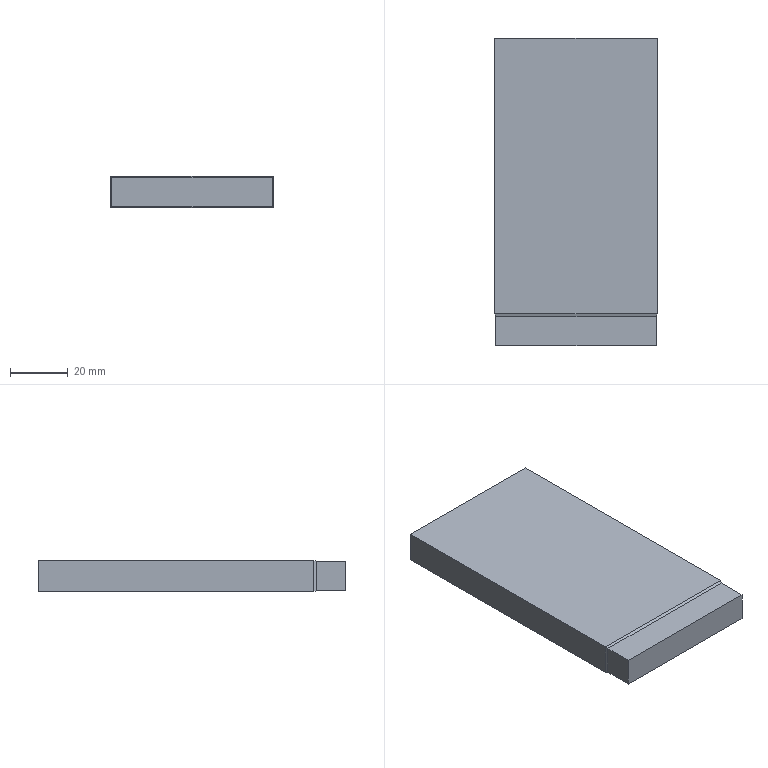Part | STEP file | 1 solid | 14 faces | box 56.208 x 106.38 x 10.782 mm | volume 63955 mm3 | plane 14
STEP:
#1=CARTESIAN_POINT('',(0.,0.,0.));
#2=DIRECTION('',(0.,0.,1.));
#3=DIRECTION('',(1.,0.,0.));
#4=AXIS2_PLACEMENT_3D('',#1,#2,#3);
#5=CARTESIAN_POINT('',(-93.931,130.5,161.754));
#6=VERTEX_POINT('',#5);
#7=CARTESIAN_POINT('',(-93.931,35.175,161.754));
#8=VERTEX_POINT('',#7);
#9=CARTESIAN_POINT('',(-93.931,185.175,161.754));
#10=DIRECTION('',(0.,-1.,0.));
#11=VECTOR('',#10,1.);
#12=LINE('',#9,#11);
#13=CARTESIAN_POINT('',(-93.931,185.175,150.972));
#14=DIRECTION('',(1.,0.,0.));
#15=DIRECTION('',(0.,0.,-1.));
#16=AXIS2_PLACEMENT_3D('',#13,#14,#15);
#17=PLANE('',#16);
#18=CARTESIAN_POINT('',(-10.782,0.));
#19=DIRECTION('',(0.,-1.));
#20=VECTOR('',#19,1.);
#21=LINE('',#18,#20);
#22=(GEOMETRIC_REPRESENTATION_CONTEXT(2)PARAMETRIC_REPRESENTATION_CONTEXT()REPRESENTATION_CONTEXT('',''));
#23=DEFINITIONAL_REPRESENTATION('',(#21),#22);
#24=PCURVE('',#17,#23);
#25=CARTESIAN_POINT('',(-65.828,185.175,161.754));
#26=DIRECTION('',(0.,0.,-1.));
#27=DIRECTION('',(-1.,0.,0.));
#28=AXIS2_PLACEMENT_3D('',#25,#26,#27);
#29=PLANE('',#28);
#30=CARTESIAN_POINT('',(28.104,0.));
#31=DIRECTION('',(0.,-1.));
#32=VECTOR('',#31,1.);
#33=LINE('',#30,#32);
#34=(GEOMETRIC_REPRESENTATION_CONTEXT(2)PARAMETRIC_REPRESENTATION_CONTEXT()REPRESENTATION_CONTEXT('',''));
#35=DEFINITIONAL_REPRESENTATION('',(#33),#34);
#36=PCURVE('',#29,#35);
#37=SURFACE_CURVE('',#12,(#24,#36),.PCURVE_S1.);
#38=EDGE_CURVE('',#6,#8,#37,.T.);
#39=ORIENTED_EDGE('',*,*,#38,.F.);
#40=CARTESIAN_POINT('',(-93.931,130.5,150.972));
#41=VERTEX_POINT('',#40);
#42=CARTESIAN_POINT('',(-93.931,130.5,150.972));
#43=DIRECTION('',(0.,0.,-1.));
#44=VECTOR('',#43,1.);
#45=LINE('',#42,#44);
#46=CARTESIAN_POINT('',(0.,-54.675));
#47=DIRECTION('',(1.,0.));
#48=VECTOR('',#47,1.);
#49=LINE('',#46,#48);
#50=(GEOMETRIC_REPRESENTATION_CONTEXT(2)PARAMETRIC_REPRESENTATION_CONTEXT()REPRESENTATION_CONTEXT('',''));
#51=DEFINITIONAL_REPRESENTATION('',(#49),#50);
#52=PCURVE('',#17,#51);
#53=CARTESIAN_POINT('',(-72.862,130.5,110.196));
#54=DIRECTION('',(0.,-1.,0.));
#55=DIRECTION('',(0.,0.,-1.));
#56=AXIS2_PLACEMENT_3D('',#53,#54,#55);
#57=PLANE('',#56);
#58=CARTESIAN_POINT('',(-40.776,-21.069));
#59=DIRECTION('',(1.,0.));
#60=VECTOR('',#59,1.);
#61=LINE('',#58,#60);
#62=(GEOMETRIC_REPRESENTATION_CONTEXT(2)PARAMETRIC_REPRESENTATION_CONTEXT()REPRESENTATION_CONTEXT('',''));
#63=DEFINITIONAL_REPRESENTATION('',(#61),#62);
#64=PCURVE('',#57,#63);
#65=SURFACE_CURVE('',#45,(#52,#64),.PCURVE_S1.);
#66=EDGE_CURVE('',#6,#41,#65,.T.);
#67=ORIENTED_EDGE('',*,*,#66,.T.);
#68=CARTESIAN_POINT('',(-93.931,35.175,150.972));
#69=VERTEX_POINT('',#68);
#70=CARTESIAN_POINT('',(-93.931,185.175,150.972));
#71=DIRECTION('',(0.,-1.,0.));
#72=VECTOR('',#71,1.);
#73=LINE('',#70,#72);
#74=CARTESIAN_POINT('',(0.,0.));
#75=DIRECTION('',(0.,-1.));
#76=VECTOR('',#75,1.);
#77=LINE('',#74,#76);
#78=(GEOMETRIC_REPRESENTATION_CONTEXT(2)PARAMETRIC_REPRESENTATION_CONTEXT()REPRESENTATION_CONTEXT('',''));
#79=DEFINITIONAL_REPRESENTATION('',(#77),#78);
#80=PCURVE('',#17,#79);
#81=CARTESIAN_POINT('',(-65.828,185.175,150.972));
#82=DIRECTION('',(0.,0.,1.));
#83=DIRECTION('',(1.,0.,0.));
#84=AXIS2_PLACEMENT_3D('',#81,#82,#83);
#85=PLANE('',#84);
#86=CARTESIAN_POINT('',(-28.104,0.));
#87=DIRECTION('',(0.,-1.));
#88=VECTOR('',#87,1.);
#89=LINE('',#86,#88);
#90=(GEOMETRIC_REPRESENTATION_CONTEXT(2)PARAMETRIC_REPRESENTATION_CONTEXT()REPRESENTATION_CONTEXT('',''));
#91=DEFINITIONAL_REPRESENTATION('',(#89),#90);
#92=PCURVE('',#85,#91);
#93=SURFACE_CURVE('',#73,(#80,#92),.PCURVE_S1.);
#94=EDGE_CURVE('',#41,#69,#93,.T.);
#95=ORIENTED_EDGE('',*,*,#94,.T.);
#96=CARTESIAN_POINT('',(-93.931,35.175,150.972));
#97=DIRECTION('',(0.,0.,1.));
#98=VECTOR('',#97,1.);
#99=LINE('',#96,#98);
#100=CARTESIAN_POINT('',(0.,-150.));
#101=DIRECTION('',(-1.,0.));
#102=VECTOR('',#101,1.);
#103=LINE('',#100,#102);
#104=(GEOMETRIC_REPRESENTATION_CONTEXT(2)PARAMETRIC_REPRESENTATION_CONTEXT()REPRESENTATION_CONTEXT('',''));
#105=DEFINITIONAL_REPRESENTATION('',(#103),#104);
#106=PCURVE('',#17,#105);
#107=CARTESIAN_POINT('',(-93.566,34.17,151.338));
#108=DIRECTION('',(-0.9397,-0.342,0.));
#109=DIRECTION('',(0.342,-0.9397,0.));
#110=AXIS2_PLACEMENT_3D('',#107,#108,#109);
#111=PLANE('',#110);
#112=CARTESIAN_POINT('',(-1.069,-0.3658));
#113=DIRECTION('',(0.,1.));
#114=VECTOR('',#113,1.);
#115=LINE('',#112,#114);
#116=(GEOMETRIC_REPRESENTATION_CONTEXT(2)PARAMETRIC_REPRESENTATION_CONTEXT()REPRESENTATION_CONTEXT('',''));
#117=DEFINITIONAL_REPRESENTATION('',(#115),#116);
#118=PCURVE('',#111,#117);
#119=SURFACE_CURVE('',#99,(#106,#118),.PCURVE_S1.);
#120=EDGE_CURVE('',#69,#8,#119,.T.);
#121=ORIENTED_EDGE('',*,*,#120,.T.);
#122=EDGE_LOOP('',(#39,#67,#95,#121));
#123=FACE_BOUND('',#122,.T.);
#124=ADVANCED_FACE('',(#123),#17,.F.);
#125=CARTESIAN_POINT('',(-37.724,130.5,161.754));
#126=VERTEX_POINT('',#125);
#127=CARTESIAN_POINT('',(-37.724,35.175,161.754));
#128=VERTEX_POINT('',#127);
#129=CARTESIAN_POINT('',(-37.724,185.175,161.754));
#130=DIRECTION('',(0.,-1.,0.));
#131=VECTOR('',#130,1.);
#132=LINE('',#129,#131);
#133=CARTESIAN_POINT('',(-28.104,0.));
#134=DIRECTION('',(0.,-1.));
#135=VECTOR('',#134,1.);
#136=LINE('',#133,#135);
#137=(GEOMETRIC_REPRESENTATION_CONTEXT(2)PARAMETRIC_REPRESENTATION_CONTEXT()REPRESENTATION_CONTEXT('',''));
#138=DEFINITIONAL_REPRESENTATION('',(#136),#137);
#139=PCURVE('',#29,#138);
#140=CARTESIAN_POINT('',(-37.724,185.175,150.972));
#141=DIRECTION('',(1.,0.,0.));
#142=DIRECTION('',(0.,0.,-1.));
#143=AXIS2_PLACEMENT_3D('',#140,#141,#142);
#144=PLANE('',#143);
#145=CARTESIAN_POINT('',(-10.782,0.));
#146=DIRECTION('',(0.,-1.));
#147=VECTOR('',#146,1.);
#148=LINE('',#145,#147);
#149=(GEOMETRIC_REPRESENTATION_CONTEXT(2)PARAMETRIC_REPRESENTATION_CONTEXT()REPRESENTATION_CONTEXT('',''));
#150=DEFINITIONAL_REPRESENTATION('',(#148),#149);
#151=PCURVE('',#144,#150);
#152=SURFACE_CURVE('',#132,(#139,#151),.PCURVE_S1.);
#153=EDGE_CURVE('',#126,#128,#152,.T.);
#154=ORIENTED_EDGE('',*,*,#153,.F.);
#155=CARTESIAN_POINT('',(-65.828,130.5,161.754));
#156=DIRECTION('',(-1.,0.,0.));
#157=VECTOR('',#156,1.);
#158=LINE('',#155,#157);
#159=CARTESIAN_POINT('',(0.,-54.675));
#160=DIRECTION('',(1.,0.));
#161=VECTOR('',#160,1.);
#162=LINE('',#159,#161);
#163=(GEOMETRIC_REPRESENTATION_CONTEXT(2)PARAMETRIC_REPRESENTATION_CONTEXT()REPRESENTATION_CONTEXT('',''));
#164=DEFINITIONAL_REPRESENTATION('',(#162),#163);
#165=PCURVE('',#29,#164);
#166=CARTESIAN_POINT('',(-51.558,7.035));
#167=DIRECTION('',(0.,-1.));
#168=VECTOR('',#167,1.);
#169=LINE('',#166,#168);
#170=(GEOMETRIC_REPRESENTATION_CONTEXT(2)PARAMETRIC_REPRESENTATION_CONTEXT()REPRESENTATION_CONTEXT('',''));
#171=DEFINITIONAL_REPRESENTATION('',(#169),#170);
#172=PCURVE('',#57,#171);
#173=SURFACE_CURVE('',#158,(#165,#172),.PCURVE_S1.);
#174=EDGE_CURVE('',#126,#6,#173,.T.);
#175=ORIENTED_EDGE('',*,*,#174,.T.);
#176=ORIENTED_EDGE('',*,*,#38,.T.);
#177=CARTESIAN_POINT('',(-65.828,35.175,161.754));
#178=DIRECTION('',(1.,0.,0.));
#179=VECTOR('',#178,1.);
#180=LINE('',#177,#179);
#181=CARTESIAN_POINT('',(0.,-150.));
#182=DIRECTION('',(-1.,0.));
#183=VECTOR('',#182,1.);
#184=LINE('',#181,#183);
#185=(GEOMETRIC_REPRESENTATION_CONTEXT(2)PARAMETRIC_REPRESENTATION_CONTEXT()REPRESENTATION_CONTEXT('',''));
#186=DEFINITIONAL_REPRESENTATION('',(#184),#185);
#187=PCURVE('',#29,#186);
#188=CARTESIAN_POINT('',(-93.566,34.17,161.388));
#189=DIRECTION('',(0.,-0.342,0.9397));
#190=DIRECTION('',(0.,-0.9397,-0.342));
#191=AXIS2_PLACEMENT_3D('',#188,#189,#190);
#192=PLANE('',#191);
#193=CARTESIAN_POINT('',(-1.069,27.738));
#194=DIRECTION('',(0.,1.));
#195=VECTOR('',#194,1.);
#196=LINE('',#193,#195);
#197=(GEOMETRIC_REPRESENTATION_CONTEXT(2)PARAMETRIC_REPRESENTATION_CONTEXT()REPRESENTATION_CONTEXT('',''));
#198=DEFINITIONAL_REPRESENTATION('',(#196),#197);
#199=PCURVE('',#192,#198);
#200=SURFACE_CURVE('',#180,(#187,#199),.PCURVE_S1.);
#201=EDGE_CURVE('',#8,#128,#200,.T.);
#202=ORIENTED_EDGE('',*,*,#201,.T.);
#203=EDGE_LOOP('',(#154,#175,#176,#202));
#204=FACE_BOUND('',#203,.T.);
#205=ADVANCED_FACE('',(#204),#29,.F.);
#206=CARTESIAN_POINT('',(-37.724,130.5,150.972));
#207=VERTEX_POINT('',#206);
#208=CARTESIAN_POINT('',(-37.724,130.5,150.972));
#209=DIRECTION('',(0.,0.,-1.));
#210=VECTOR('',#209,1.);
#211=LINE('',#208,#210);
#212=CARTESIAN_POINT('',(0.,-54.675));
#213=DIRECTION('',(1.,0.));
#214=VECTOR('',#213,1.);
#215=LINE('',#212,#214);
#216=(GEOMETRIC_REPRESENTATION_CONTEXT(2)PARAMETRIC_REPRESENTATION_CONTEXT()REPRESENTATION_CONTEXT('',''));
#217=DEFINITIONAL_REPRESENTATION('',(#215),#216);
#218=PCURVE('',#144,#217);
#219=CARTESIAN_POINT('',(-40.776,35.139));
#220=DIRECTION('',(1.,0.));
#221=VECTOR('',#220,1.);
#222=LINE('',#219,#221);
#223=(GEOMETRIC_REPRESENTATION_CONTEXT(2)PARAMETRIC_REPRESENTATION_CONTEXT()REPRESENTATION_CONTEXT('',''));
#224=DEFINITIONAL_REPRESENTATION('',(#222),#223);
#225=PCURVE('',#57,#224);
#226=SURFACE_CURVE('',#211,(#218,#225),.PCURVE_S1.);
#227=EDGE_CURVE('',#126,#207,#226,.T.);
#228=ORIENTED_EDGE('',*,*,#227,.F.);
#229=ORIENTED_EDGE('',*,*,#153,.T.);
#230=CARTESIAN_POINT('',(-37.724,35.175,150.972));
#231=VERTEX_POINT('',#230);
#232=CARTESIAN_POINT('',(-37.724,35.175,150.972));
#233=DIRECTION('',(0.,0.,1.));
#234=VECTOR('',#233,1.);
#235=LINE('',#232,#234);
#236=CARTESIAN_POINT('',(0.,-150.));
#237=DIRECTION('',(-1.,0.));
#238=VECTOR('',#237,1.);
#239=LINE('',#236,#238);
#240=(GEOMETRIC_REPRESENTATION_CONTEXT(2)PARAMETRIC_REPRESENTATION_CONTEXT()REPRESENTATION_CONTEXT('',''));
#241=DEFINITIONAL_REPRESENTATION('',(#239),#240);
#242=PCURVE('',#144,#241);
#243=CARTESIAN_POINT('',(-38.09,34.17,151.338));
#244=DIRECTION('',(0.9397,-0.342,0.));
#245=DIRECTION('',(0.342,0.9397,0.));
#246=AXIS2_PLACEMENT_3D('',#243,#244,#245);
#247=PLANE('',#246);
#248=CARTESIAN_POINT('',(1.069,-0.3658));
#249=DIRECTION('',(0.,1.));
#250=VECTOR('',#249,1.);
#251=LINE('',#248,#250);
#252=(GEOMETRIC_REPRESENTATION_CONTEXT(2)PARAMETRIC_REPRESENTATION_CONTEXT()REPRESENTATION_CONTEXT('',''));
#253=DEFINITIONAL_REPRESENTATION('',(#251),#252);
#254=PCURVE('',#247,#253);
#255=SURFACE_CURVE('',#235,(#242,#254),.PCURVE_S1.);
#256=EDGE_CURVE('',#231,#128,#255,.T.);
#257=ORIENTED_EDGE('',*,*,#256,.F.);
#258=CARTESIAN_POINT('',(-37.724,185.175,150.972));
#259=DIRECTION('',(0.,-1.,0.));
#260=VECTOR('',#259,1.);
#261=LINE('',#258,#260);
#262=CARTESIAN_POINT('',(0.,0.));
#263=DIRECTION('',(0.,-1.));
#264=VECTOR('',#263,1.);
#265=LINE('',#262,#264);
#266=(GEOMETRIC_REPRESENTATION_CONTEXT(2)PARAMETRIC_REPRESENTATION_CONTEXT()REPRESENTATION_CONTEXT('',''));
#267=DEFINITIONAL_REPRESENTATION('',(#265),#266);
#268=PCURVE('',#144,#267);
#269=CARTESIAN_POINT('',(28.104,0.));
#270=DIRECTION('',(0.,-1.));
#271=VECTOR('',#270,1.);
#272=LINE('',#269,#271);
#273=(GEOMETRIC_REPRESENTATION_CONTEXT(2)PARAMETRIC_REPRESENTATION_CONTEXT()REPRESENTATION_CONTEXT('',''));
#274=DEFINITIONAL_REPRESENTATION('',(#272),#273);
#275=PCURVE('',#85,#274);
#276=SURFACE_CURVE('',#261,(#268,#275),.PCURVE_S1.);
#277=EDGE_CURVE('',#207,#231,#276,.T.);
#278=ORIENTED_EDGE('',*,*,#277,.F.);
#279=EDGE_LOOP('',(#228,#229,#257,#278));
#280=FACE_BOUND('',#279,.T.);
#281=ADVANCED_FACE('',(#280),#144,.T.);
#282=ORIENTED_EDGE('',*,*,#94,.F.);
#283=CARTESIAN_POINT('',(-65.828,130.5,150.972));
#284=DIRECTION('',(1.,0.,0.));
#285=VECTOR('',#284,1.);
#286=LINE('',#283,#285);
#287=CARTESIAN_POINT('',(0.,-54.675));
#288=DIRECTION('',(1.,0.));
#289=VECTOR('',#288,1.);
#290=LINE('',#287,#289);
#291=(GEOMETRIC_REPRESENTATION_CONTEXT(2)PARAMETRIC_REPRESENTATION_CONTEXT()REPRESENTATION_CONTEXT('',''));
#292=DEFINITIONAL_REPRESENTATION('',(#290),#291);
#293=PCURVE('',#85,#292);
#294=CARTESIAN_POINT('',(-40.776,7.035));
#295=DIRECTION('',(0.,1.));
#296=VECTOR('',#295,1.);
#297=LINE('',#294,#296);
#298=(GEOMETRIC_REPRESENTATION_CONTEXT(2)PARAMETRIC_REPRESENTATION_CONTEXT()REPRESENTATION_CONTEXT('',''));
#299=DEFINITIONAL_REPRESENTATION('',(#297),#298);
#300=PCURVE('',#57,#299);
#301=SURFACE_CURVE('',#286,(#293,#300),.PCURVE_S1.);
#302=EDGE_CURVE('',#41,#207,#301,.T.);
#303=ORIENTED_EDGE('',*,*,#302,.T.);
#304=ORIENTED_EDGE('',*,*,#277,.T.);
#305=CARTESIAN_POINT('',(-65.828,35.175,150.972));
#306=DIRECTION('',(-1.,0.,0.));
#307=VECTOR('',#306,1.);
#308=LINE('',#305,#307);
#309=CARTESIAN_POINT('',(0.,-150.));
#310=DIRECTION('',(-1.,0.));
#311=VECTOR('',#310,1.);
#312=LINE('',#309,#311);
#313=(GEOMETRIC_REPRESENTATION_CONTEXT(2)PARAMETRIC_REPRESENTATION_CONTEXT()REPRESENTATION_CONTEXT('',''));
#314=DEFINITIONAL_REPRESENTATION('',(#312),#313);
#315=PCURVE('',#85,#314);
#316=CARTESIAN_POINT('',(-93.566,34.17,151.338));
#317=DIRECTION('',(0.,-0.342,-0.9397));
#318=DIRECTION('',(0.,0.9397,-0.342));
#319=AXIS2_PLACEMENT_3D('',#316,#317,#318);
#320=PLANE('',#319);
#321=CARTESIAN_POINT('',(1.069,27.738));
#322=DIRECTION('',(0.,-1.));
#323=VECTOR('',#322,1.);
#324=LINE('',#321,#323);
#325=(GEOMETRIC_REPRESENTATION_CONTEXT(2)PARAMETRIC_REPRESENTATION_CONTEXT()REPRESENTATION_CONTEXT('',''));
#326=DEFINITIONAL_REPRESENTATION('',(#324),#325);
#327=PCURVE('',#320,#326);
#328=SURFACE_CURVE('',#308,(#315,#327),.PCURVE_S1.);
#329=EDGE_CURVE('',#231,#69,#328,.T.);
#330=ORIENTED_EDGE('',*,*,#329,.T.);
#331=EDGE_LOOP('',(#282,#303,#304,#330));
#332=FACE_BOUND('',#331,.T.);
#333=ADVANCED_FACE('',(#332),#85,.F.);
#334=CARTESIAN_POINT('',(-38.09,24.12,151.338));
#335=VERTEX_POINT('',#334);
#336=CARTESIAN_POINT('',(-38.09,24.12,161.388));
#337=VERTEX_POINT('',#336);
#338=CARTESIAN_POINT('',(-38.09,24.12,161.388));
#339=DIRECTION('',(0.,0.,1.));
#340=VECTOR('',#339,1.);
#341=LINE('',#338,#340);
#342=CARTESIAN_POINT('',(-65.828,24.12,150.972));
#343=DIRECTION('',(0.,-1.,0.));
#344=DIRECTION('',(0.,0.,-1.));
#345=AXIS2_PLACEMENT_3D('',#342,#343,#344);
#346=PLANE('',#345);
#347=CARTESIAN_POINT('',(-10.416,27.738));
#348=DIRECTION('',(-1.,0.));
#349=VECTOR('',#348,1.);
#350=LINE('',#347,#349);
#351=(GEOMETRIC_REPRESENTATION_CONTEXT(2)PARAMETRIC_REPRESENTATION_CONTEXT()REPRESENTATION_CONTEXT('',''));
#352=DEFINITIONAL_REPRESENTATION('',(#350),#351);
#353=PCURVE('',#346,#352);
#354=CARTESIAN_POINT('',(-38.09,24.12,151.338));
#355=DIRECTION('',(1.,0.,0.));
#356=DIRECTION('',(0.,0.,-1.));
#357=AXIS2_PLACEMENT_3D('',#354,#355,#356);
#358=PLANE('',#357);
#359=CARTESIAN_POINT('',(-10.05,0.));
#360=DIRECTION('',(-1.,0.));
#361=VECTOR('',#360,1.);
#362=LINE('',#359,#361);
#363=(GEOMETRIC_REPRESENTATION_CONTEXT(2)PARAMETRIC_REPRESENTATION_CONTEXT()REPRESENTATION_CONTEXT('',''));
#364=DEFINITIONAL_REPRESENTATION('',(#362),#363);
#365=PCURVE('',#358,#364);
#366=SURFACE_CURVE('',#341,(#353,#365),.PCURVE_S1.);
#367=EDGE_CURVE('',#335,#337,#366,.T.);
#368=ORIENTED_EDGE('',*,*,#367,.T.);
#369=CARTESIAN_POINT('',(-93.566,24.12,161.388));
#370=VERTEX_POINT('',#369);
#371=CARTESIAN_POINT('',(-93.566,24.12,161.388));
#372=DIRECTION('',(-1.,0.,0.));
#373=VECTOR('',#372,1.);
#374=LINE('',#371,#373);
#375=CARTESIAN_POINT('',(-10.416,-27.738));
#376=DIRECTION('',(0.,-1.));
#377=VECTOR('',#376,1.);
#378=LINE('',#375,#377);
#379=(GEOMETRIC_REPRESENTATION_CONTEXT(2)PARAMETRIC_REPRESENTATION_CONTEXT()REPRESENTATION_CONTEXT('',''));
#380=DEFINITIONAL_REPRESENTATION('',(#378),#379);
#381=PCURVE('',#346,#380);
#382=CARTESIAN_POINT('',(-93.566,24.12,161.388));
#383=DIRECTION('',(0.,0.,1.));
#384=DIRECTION('',(0.,-1.,0.));
#385=AXIS2_PLACEMENT_3D('',#382,#383,#384);
#386=PLANE('',#385);
#387=CARTESIAN_POINT('',(0.,0.));
#388=DIRECTION('',(0.,-1.));
#389=VECTOR('',#388,1.);
#390=LINE('',#387,#389);
#391=(GEOMETRIC_REPRESENTATION_CONTEXT(2)PARAMETRIC_REPRESENTATION_CONTEXT()REPRESENTATION_CONTEXT('',''));
#392=DEFINITIONAL_REPRESENTATION('',(#390),#391);
#393=PCURVE('',#386,#392);
#394=SURFACE_CURVE('',#374,(#381,#393),.PCURVE_S1.);
#395=EDGE_CURVE('',#337,#370,#394,.T.);
#396=ORIENTED_EDGE('',*,*,#395,.T.);
#397=CARTESIAN_POINT('',(-93.566,24.12,151.338));
#398=VERTEX_POINT('',#397);
#399=CARTESIAN_POINT('',(-93.566,24.12,151.338));
#400=DIRECTION('',(0.,0.,-1.));
#401=VECTOR('',#400,1.);
#402=LINE('',#399,#401);
#403=CARTESIAN_POINT('',(-0.3658,-27.738));
#404=DIRECTION('',(1.,0.));
#405=VECTOR('',#404,1.);
#406=LINE('',#403,#405);
#407=(GEOMETRIC_REPRESENTATION_CONTEXT(2)PARAMETRIC_REPRESENTATION_CONTEXT()REPRESENTATION_CONTEXT('',''));
#408=DEFINITIONAL_REPRESENTATION('',(#406),#407);
#409=PCURVE('',#346,#408);
#410=CARTESIAN_POINT('',(-93.566,24.12,151.338));
#411=DIRECTION('',(-1.,0.,0.));
#412=DIRECTION('',(0.,-1.,0.));
#413=AXIS2_PLACEMENT_3D('',#410,#411,#412);
#414=PLANE('',#413);
#415=CARTESIAN_POINT('',(0.,0.));
#416=DIRECTION('',(0.,-1.));
#417=VECTOR('',#416,1.);
#418=LINE('',#415,#417);
#419=(GEOMETRIC_REPRESENTATION_CONTEXT(2)PARAMETRIC_REPRESENTATION_CONTEXT()REPRESENTATION_CONTEXT('',''));
#420=DEFINITIONAL_REPRESENTATION('',(#418),#419);
#421=PCURVE('',#414,#420);
#422=SURFACE_CURVE('',#402,(#409,#421),.PCURVE_S1.);
#423=EDGE_CURVE('',#370,#398,#422,.T.);
#424=ORIENTED_EDGE('',*,*,#423,.T.);
#425=CARTESIAN_POINT('',(-38.09,24.12,151.338));
#426=DIRECTION('',(1.,0.,0.));
#427=VECTOR('',#426,1.);
#428=LINE('',#425,#427);
#429=CARTESIAN_POINT('',(-0.3658,27.738));
#430=DIRECTION('',(0.,1.));
#431=VECTOR('',#430,1.);
#432=LINE('',#429,#431);
#433=(GEOMETRIC_REPRESENTATION_CONTEXT(2)PARAMETRIC_REPRESENTATION_CONTEXT()REPRESENTATION_CONTEXT('',''));
#434=DEFINITIONAL_REPRESENTATION('',(#432),#433);
#435=PCURVE('',#346,#434);
#436=CARTESIAN_POINT('',(-93.566,24.12,151.338));
#437=DIRECTION('',(0.,0.,-1.));
#438=DIRECTION('',(-1.,0.,0.));
#439=AXIS2_PLACEMENT_3D('',#436,#437,#438);
#440=PLANE('',#439);
#441=CARTESIAN_POINT('',(-55.476,0.));
#442=DIRECTION('',(-1.,0.));
#443=VECTOR('',#442,1.);
#444=LINE('',#441,#443);
#445=(GEOMETRIC_REPRESENTATION_CONTEXT(2)PARAMETRIC_REPRESENTATION_CONTEXT()REPRESENTATION_CONTEXT('',''));
#446=DEFINITIONAL_REPRESENTATION('',(#444),#445);
#447=PCURVE('',#440,#446);
#448=SURFACE_CURVE('',#428,(#435,#447),.PCURVE_S1.);
#449=EDGE_CURVE('',#398,#335,#448,.T.);
#450=ORIENTED_EDGE('',*,*,#449,.T.);
#451=EDGE_LOOP('',(#368,#396,#424,#450));
#452=FACE_BOUND('',#451,.T.);
#453=ADVANCED_FACE('',(#452),#346,.T.);
#454=CARTESIAN_POINT('',(-38.09,34.17,161.388));
#455=VERTEX_POINT('',#454);
#456=CARTESIAN_POINT('',(-38.09,24.12,161.388));
#457=DIRECTION('',(0.,1.,0.));
#458=VECTOR('',#457,1.);
#459=LINE('',#456,#458);
#460=CARTESIAN_POINT('',(-10.05,0.));
#461=DIRECTION('',(0.,1.));
#462=VECTOR('',#461,1.);
#463=LINE('',#460,#462);
#464=(GEOMETRIC_REPRESENTATION_CONTEXT(2)PARAMETRIC_REPRESENTATION_CONTEXT()REPRESENTATION_CONTEXT('',''));
#465=DEFINITIONAL_REPRESENTATION('',(#463),#464);
#466=PCURVE('',#358,#465);
#467=CARTESIAN_POINT('',(0.,55.476));
#468=DIRECTION('',(-1.,0.));
#469=VECTOR('',#468,1.);
#470=LINE('',#467,#469);
#471=(GEOMETRIC_REPRESENTATION_CONTEXT(2)PARAMETRIC_REPRESENTATION_CONTEXT()REPRESENTATION_CONTEXT('',''));
#472=DEFINITIONAL_REPRESENTATION('',(#470),#471);
#473=PCURVE('',#386,#472);
#474=SURFACE_CURVE('',#459,(#466,#473),.PCURVE_S1.);
#475=EDGE_CURVE('',#337,#455,#474,.T.);
#476=ORIENTED_EDGE('',*,*,#475,.F.);
#477=ORIENTED_EDGE('',*,*,#367,.F.);
#478=CARTESIAN_POINT('',(-38.09,34.17,151.338));
#479=VERTEX_POINT('',#478);
#480=CARTESIAN_POINT('',(-38.09,24.12,151.338));
#481=DIRECTION('',(0.,1.,0.));
#482=VECTOR('',#481,1.);
#483=LINE('',#480,#482);
#484=CARTESIAN_POINT('',(0.,0.));
#485=DIRECTION('',(0.,1.));
#486=VECTOR('',#485,1.);
#487=LINE('',#484,#486);
#488=(GEOMETRIC_REPRESENTATION_CONTEXT(2)PARAMETRIC_REPRESENTATION_CONTEXT()REPRESENTATION_CONTEXT('',''));
#489=DEFINITIONAL_REPRESENTATION('',(#487),#488);
#490=PCURVE('',#358,#489);
#491=CARTESIAN_POINT('',(-55.476,0.));
#492=DIRECTION('',(0.,1.));
#493=VECTOR('',#492,1.);
#494=LINE('',#491,#493);
#495=(GEOMETRIC_REPRESENTATION_CONTEXT(2)PARAMETRIC_REPRESENTATION_CONTEXT()REPRESENTATION_CONTEXT('',''));
#496=DEFINITIONAL_REPRESENTATION('',(#494),#495);
#497=PCURVE('',#440,#496);
#498=SURFACE_CURVE('',#483,(#490,#497),.PCURVE_S1.);
#499=EDGE_CURVE('',#335,#479,#498,.T.);
#500=ORIENTED_EDGE('',*,*,#499,.T.);
#501=CARTESIAN_POINT('',(-38.09,34.17,151.338));
#502=DIRECTION('',(0.,0.,-1.));
#503=VECTOR('',#502,1.);
#504=LINE('',#501,#503);
#505=CARTESIAN_POINT('',(0.,10.05));
#506=DIRECTION('',(1.,0.));
#507=VECTOR('',#506,1.);
#508=LINE('',#505,#507);
#509=(GEOMETRIC_REPRESENTATION_CONTEXT(2)PARAMETRIC_REPRESENTATION_CONTEXT()REPRESENTATION_CONTEXT('',''));
#510=DEFINITIONAL_REPRESENTATION('',(#508),#509);
#511=PCURVE('',#358,#510);
#512=CARTESIAN_POINT('',(0.,0.));
#513=DIRECTION('',(0.,-1.));
#514=VECTOR('',#513,1.);
#515=LINE('',#512,#514);
#516=(GEOMETRIC_REPRESENTATION_CONTEXT(2)PARAMETRIC_REPRESENTATION_CONTEXT()REPRESENTATION_CONTEXT('',''));
#517=DEFINITIONAL_REPRESENTATION('',(#515),#516);
#518=PCURVE('',#247,#517);
#519=SURFACE_CURVE('',#504,(#511,#518),.PCURVE_S1.);
#520=EDGE_CURVE('',#455,#479,#519,.T.);
#521=ORIENTED_EDGE('',*,*,#520,.F.);
#522=EDGE_LOOP('',(#476,#477,#500,#521));
#523=FACE_BOUND('',#522,.T.);
#524=ADVANCED_FACE('',(#523),#358,.T.);
#525=CARTESIAN_POINT('',(-43.899,18.208,155.578));
#526=DIRECTION('',(-0.3236,-0.8891,-0.3236));
#527=VECTOR('',#526,1.);
#528=LINE('',#525,#527);
#529=CARTESIAN_POINT('',(-16.987,4.24));
#530=DIRECTION('',(-0.9462,-0.3236));
#531=VECTOR('',#530,1.);
#532=LINE('',#529,#531);
#533=(GEOMETRIC_REPRESENTATION_CONTEXT(2)PARAMETRIC_REPRESENTATION_CONTEXT()REPRESENTATION_CONTEXT('',''));
#534=DEFINITIONAL_REPRESENTATION('',(#532),#533);
#535=PCURVE('',#247,#534);
#536=CARTESIAN_POINT('',(16.987,49.666));
#537=DIRECTION('',(0.9462,-0.3236));
#538=VECTOR('',#537,1.);
#539=LINE('',#536,#538);
#540=(GEOMETRIC_REPRESENTATION_CONTEXT(2)PARAMETRIC_REPRESENTATION_CONTEXT()REPRESENTATION_CONTEXT('',''));
#541=DEFINITIONAL_REPRESENTATION('',(#539),#540);
#542=PCURVE('',#192,#541);
#543=SURFACE_CURVE('',#528,(#535,#542),.PCURVE_S1.);
#544=EDGE_CURVE('',#128,#455,#543,.T.);
#545=ORIENTED_EDGE('',*,*,#544,.T.);
#546=ORIENTED_EDGE('',*,*,#520,.T.);
#547=CARTESIAN_POINT('',(-38.09,34.17,151.338));
#548=DIRECTION('',(0.3236,0.8891,-0.3236));
#549=VECTOR('',#548,1.);
#550=LINE('',#547,#549);
#551=CARTESIAN_POINT('',(0.,0.));
#552=DIRECTION('',(0.9462,-0.3236));
#553=VECTOR('',#552,1.);
#554=LINE('',#551,#553);
#555=(GEOMETRIC_REPRESENTATION_CONTEXT(2)PARAMETRIC_REPRESENTATION_CONTEXT()REPRESENTATION_CONTEXT('',''));
#556=DEFINITIONAL_REPRESENTATION('',(#554),#555);
#557=PCURVE('',#247,#556);
#558=CARTESIAN_POINT('',(0.,55.476));
#559=DIRECTION('',(0.9462,0.3236));
#560=VECTOR('',#559,1.);
#561=LINE('',#558,#560);
#562=(GEOMETRIC_REPRESENTATION_CONTEXT(2)PARAMETRIC_REPRESENTATION_CONTEXT()REPRESENTATION_CONTEXT('',''));
#563=DEFINITIONAL_REPRESENTATION('',(#561),#562);
#564=PCURVE('',#320,#563);
#565=SURFACE_CURVE('',#550,(#557,#564),.PCURVE_S1.);
#566=EDGE_CURVE('',#479,#231,#565,.T.);
#567=ORIENTED_EDGE('',*,*,#566,.T.);
#568=ORIENTED_EDGE('',*,*,#256,.T.);
#569=EDGE_LOOP('',(#545,#546,#567,#568));
#570=FACE_BOUND('',#569,.T.);
#571=ADVANCED_FACE('',(#570),#247,.T.);
#572=ORIENTED_EDGE('',*,*,#201,.F.);
#573=CARTESIAN_POINT('',(-93.566,34.17,161.388));
#574=VERTEX_POINT('',#573);
#575=CARTESIAN_POINT('',(-92.513,31.278,160.335));
#576=DIRECTION('',(0.3236,-0.8891,-0.3236));
#577=VECTOR('',#576,1.);
#578=LINE('',#575,#577);
#579=CARTESIAN_POINT('',(3.077,1.053));
#580=DIRECTION('',(0.9462,0.3236));
#581=VECTOR('',#580,1.);
#582=LINE('',#579,#581);
#583=(GEOMETRIC_REPRESENTATION_CONTEXT(2)PARAMETRIC_REPRESENTATION_CONTEXT()REPRESENTATION_CONTEXT('',''));
#584=DEFINITIONAL_REPRESENTATION('',(#582),#583);
#585=PCURVE('',#192,#584);
#586=CARTESIAN_POINT('',(3.077,8.997));
#587=DIRECTION('',(0.9462,-0.3236));
#588=VECTOR('',#587,1.);
#589=LINE('',#586,#588);
#590=(GEOMETRIC_REPRESENTATION_CONTEXT(2)PARAMETRIC_REPRESENTATION_CONTEXT()REPRESENTATION_CONTEXT('',''));
#591=DEFINITIONAL_REPRESENTATION('',(#589),#590);
#592=PCURVE('',#111,#591);
#593=SURFACE_CURVE('',#578,(#585,#592),.PCURVE_S1.);
#594=EDGE_CURVE('',#8,#574,#593,.T.);
#595=ORIENTED_EDGE('',*,*,#594,.T.);
#596=CARTESIAN_POINT('',(-93.566,34.17,161.388));
#597=DIRECTION('',(1.,0.,0.));
#598=VECTOR('',#597,1.);
#599=LINE('',#596,#598);
#600=CARTESIAN_POINT('',(0.,0.));
#601=DIRECTION('',(0.,1.));
#602=VECTOR('',#601,1.);
#603=LINE('',#600,#602);
#604=(GEOMETRIC_REPRESENTATION_CONTEXT(2)PARAMETRIC_REPRESENTATION_CONTEXT()REPRESENTATION_CONTEXT('',''));
#605=DEFINITIONAL_REPRESENTATION('',(#603),#604);
#606=PCURVE('',#192,#605);
#607=CARTESIAN_POINT('',(-10.05,0.));
#608=DIRECTION('',(0.,1.));
#609=VECTOR('',#608,1.);
#610=LINE('',#607,#609);
#611=(GEOMETRIC_REPRESENTATION_CONTEXT(2)PARAMETRIC_REPRESENTATION_CONTEXT()REPRESENTATION_CONTEXT('',''));
#612=DEFINITIONAL_REPRESENTATION('',(#610),#611);
#613=PCURVE('',#386,#612);
#614=SURFACE_CURVE('',#599,(#606,#613),.PCURVE_S1.);
#615=EDGE_CURVE('',#574,#455,#614,.T.);
#616=ORIENTED_EDGE('',*,*,#615,.T.);
#617=ORIENTED_EDGE('',*,*,#544,.F.);
#618=EDGE_LOOP('',(#572,#595,#616,#617));
#619=FACE_BOUND('',#618,.T.);
#620=ADVANCED_FACE('',(#619),#192,.T.);
#621=ORIENTED_EDGE('',*,*,#615,.F.);
#622=CARTESIAN_POINT('',(-93.566,24.12,161.388));
#623=DIRECTION('',(0.,1.,0.));
#624=VECTOR('',#623,1.);
#625=LINE('',#622,#624);
#626=CARTESIAN_POINT('',(0.,0.));
#627=DIRECTION('',(-1.,0.));
#628=VECTOR('',#627,1.);
#629=LINE('',#626,#628);
#630=(GEOMETRIC_REPRESENTATION_CONTEXT(2)PARAMETRIC_REPRESENTATION_CONTEXT()REPRESENTATION_CONTEXT('',''));
#631=DEFINITIONAL_REPRESENTATION('',(#629),#630);
#632=PCURVE('',#386,#631);
#633=CARTESIAN_POINT('',(0.,10.05));
#634=DIRECTION('',(-1.,0.));
#635=VECTOR('',#634,1.);
#636=LINE('',#633,#635);
#637=(GEOMETRIC_REPRESENTATION_CONTEXT(2)PARAMETRIC_REPRESENTATION_CONTEXT()REPRESENTATION_CONTEXT('',''));
#638=DEFINITIONAL_REPRESENTATION('',(#636),#637);
#639=PCURVE('',#414,#638);
#640=SURFACE_CURVE('',#625,(#632,#639),.PCURVE_S1.);
#641=EDGE_CURVE('',#370,#574,#640,.T.);
#642=ORIENTED_EDGE('',*,*,#641,.F.);
#643=ORIENTED_EDGE('',*,*,#395,.F.);
#644=ORIENTED_EDGE('',*,*,#475,.T.);
#645=EDGE_LOOP('',(#621,#642,#643,#644));
#646=FACE_BOUND('',#645,.T.);
#647=ADVANCED_FACE('',(#646),#386,.T.);
#648=ORIENTED_EDGE('',*,*,#449,.F.);
#649=CARTESIAN_POINT('',(-93.566,34.17,151.338));
#650=VERTEX_POINT('',#649);
#651=CARTESIAN_POINT('',(-93.566,24.12,151.338));
#652=DIRECTION('',(0.,1.,0.));
#653=VECTOR('',#652,1.);
#654=LINE('',#651,#653);
#655=CARTESIAN_POINT('',(0.,0.));
#656=DIRECTION('',(0.,1.));
#657=VECTOR('',#656,1.);
#658=LINE('',#655,#657);
#659=(GEOMETRIC_REPRESENTATION_CONTEXT(2)PARAMETRIC_REPRESENTATION_CONTEXT()REPRESENTATION_CONTEXT('',''));
#660=DEFINITIONAL_REPRESENTATION('',(#658),#659);
#661=PCURVE('',#440,#660);
#662=CARTESIAN_POINT('',(0.,0.));
#663=DIRECTION('',(-1.,0.));
#664=VECTOR('',#663,1.);
#665=LINE('',#662,#664);
#666=(GEOMETRIC_REPRESENTATION_CONTEXT(2)PARAMETRIC_REPRESENTATION_CONTEXT()REPRESENTATION_CONTEXT('',''));
#667=DEFINITIONAL_REPRESENTATION('',(#665),#666);
#668=PCURVE('',#414,#667);
#669=SURFACE_CURVE('',#654,(#661,#668),.PCURVE_S1.);
#670=EDGE_CURVE('',#398,#650,#669,.T.);
#671=ORIENTED_EDGE('',*,*,#670,.T.);
#672=CARTESIAN_POINT('',(-93.566,34.17,151.338));
#673=DIRECTION('',(-1.,0.,0.));
#674=VECTOR('',#673,1.);
#675=LINE('',#672,#674);
#676=CARTESIAN_POINT('',(0.,10.05));
#677=DIRECTION('',(1.,0.));
#678=VECTOR('',#677,1.);
#679=LINE('',#676,#678);
#680=(GEOMETRIC_REPRESENTATION_CONTEXT(2)PARAMETRIC_REPRESENTATION_CONTEXT()REPRESENTATION_CONTEXT('',''));
#681=DEFINITIONAL_REPRESENTATION('',(#679),#680);
#682=PCURVE('',#440,#681);
#683=CARTESIAN_POINT('',(0.,0.));
#684=DIRECTION('',(0.,-1.));
#685=VECTOR('',#684,1.);
#686=LINE('',#683,#685);
#687=(GEOMETRIC_REPRESENTATION_CONTEXT(2)PARAMETRIC_REPRESENTATION_CONTEXT()REPRESENTATION_CONTEXT('',''));
#688=DEFINITIONAL_REPRESENTATION('',(#686),#687);
#689=PCURVE('',#320,#688);
#690=SURFACE_CURVE('',#675,(#682,#689),.PCURVE_S1.);
#691=EDGE_CURVE('',#479,#650,#690,.T.);
#692=ORIENTED_EDGE('',*,*,#691,.F.);
#693=ORIENTED_EDGE('',*,*,#499,.F.);
#694=EDGE_LOOP('',(#648,#671,#692,#693));
#695=FACE_BOUND('',#694,.T.);
#696=ADVANCED_FACE('',(#695),#440,.T.);
#697=ORIENTED_EDGE('',*,*,#691,.T.);
#698=CARTESIAN_POINT('',(-93.566,34.17,151.338));
#699=DIRECTION('',(-0.3236,0.8891,-0.3236));
#700=VECTOR('',#699,1.);
#701=LINE('',#698,#700);
#702=CARTESIAN_POINT('',(0.,0.));
#703=DIRECTION('',(0.9462,-0.3236));
#704=VECTOR('',#703,1.);
#705=LINE('',#702,#704);
#706=(GEOMETRIC_REPRESENTATION_CONTEXT(2)PARAMETRIC_REPRESENTATION_CONTEXT()REPRESENTATION_CONTEXT('',''));
#707=DEFINITIONAL_REPRESENTATION('',(#705),#706);
#708=PCURVE('',#320,#707);
#709=CARTESIAN_POINT('',(0.,0.));
#710=DIRECTION('',(-0.9462,-0.3236));
#711=VECTOR('',#710,1.);
#712=LINE('',#709,#711);
#713=(GEOMETRIC_REPRESENTATION_CONTEXT(2)PARAMETRIC_REPRESENTATION_CONTEXT()REPRESENTATION_CONTEXT('',''));
#714=DEFINITIONAL_REPRESENTATION('',(#712),#713);
#715=PCURVE('',#111,#714);
#716=SURFACE_CURVE('',#701,(#708,#715),.PCURVE_S1.);
#717=EDGE_CURVE('',#650,#69,#716,.T.);
#718=ORIENTED_EDGE('',*,*,#717,.T.);
#719=ORIENTED_EDGE('',*,*,#329,.F.);
#720=ORIENTED_EDGE('',*,*,#566,.F.);
#721=EDGE_LOOP('',(#697,#718,#719,#720));
#722=FACE_BOUND('',#721,.T.);
#723=ADVANCED_FACE('',(#722),#320,.T.);
#724=ORIENTED_EDGE('',*,*,#670,.F.);
#725=ORIENTED_EDGE('',*,*,#423,.F.);
#726=ORIENTED_EDGE('',*,*,#641,.T.);
#727=CARTESIAN_POINT('',(-93.566,34.17,151.338));
#728=DIRECTION('',(0.,0.,1.));
#729=VECTOR('',#728,1.);
#730=LINE('',#727,#729);
#731=CARTESIAN_POINT('',(-10.05,0.));
#732=DIRECTION('',(0.,1.));
#733=VECTOR('',#732,1.);
#734=LINE('',#731,#733);
#735=(GEOMETRIC_REPRESENTATION_CONTEXT(2)PARAMETRIC_REPRESENTATION_CONTEXT()REPRESENTATION_CONTEXT('',''));
#736=DEFINITIONAL_REPRESENTATION('',(#734),#735);
#737=PCURVE('',#414,#736);
#738=CARTESIAN_POINT('',(0.,0.));
#739=DIRECTION('',(0.,1.));
#740=VECTOR('',#739,1.);
#741=LINE('',#738,#740);
#742=(GEOMETRIC_REPRESENTATION_CONTEXT(2)PARAMETRIC_REPRESENTATION_CONTEXT()REPRESENTATION_CONTEXT('',''));
#743=DEFINITIONAL_REPRESENTATION('',(#741),#742);
#744=PCURVE('',#111,#743);
#745=SURFACE_CURVE('',#730,(#737,#744),.PCURVE_S1.);
#746=EDGE_CURVE('',#650,#574,#745,.T.);
#747=ORIENTED_EDGE('',*,*,#746,.F.);
#748=EDGE_LOOP('',(#724,#725,#726,#747));
#749=FACE_BOUND('',#748,.T.);
#750=ADVANCED_FACE('',(#749),#414,.T.);
#751=ORIENTED_EDGE('',*,*,#717,.F.);
#752=ORIENTED_EDGE('',*,*,#746,.T.);
#753=ORIENTED_EDGE('',*,*,#594,.F.);
#754=ORIENTED_EDGE('',*,*,#120,.F.);
#755=EDGE_LOOP('',(#751,#752,#753,#754));
#756=FACE_BOUND('',#755,.T.);
#757=ADVANCED_FACE('',(#756),#111,.T.);
#758=ORIENTED_EDGE('',*,*,#66,.F.);
#759=ORIENTED_EDGE('',*,*,#174,.F.);
#760=ORIENTED_EDGE('',*,*,#227,.T.);
#761=ORIENTED_EDGE('',*,*,#302,.F.);
#762=EDGE_LOOP('',(#758,#759,#760,#761));
#763=FACE_BOUND('',#762,.T.);
#764=ADVANCED_FACE('',(#763),#57,.F.);
#765=CLOSED_SHELL('',(#124,#205,#281,#333,#453,#524,#571,#620,#647,#696,#723,#750,#757,#764));
#766=MANIFOLD_SOLID_BREP('',#765);
#767=(LENGTH_UNIT()NAMED_UNIT(*)SI_UNIT(.MILLI.,.METRE.));
#768=UNCERTAINTY_MEASURE_WITH_UNIT(LENGTH_MEASURE(0.0000001),#767,'','');
#769=(NAMED_UNIT(*)PLANE_ANGLE_UNIT()SI_UNIT($,.RADIAN.));
#770=(NAMED_UNIT(*)SI_UNIT($,.STERADIAN.)SOLID_ANGLE_UNIT());
#771=(GEOMETRIC_REPRESENTATION_CONTEXT(3)GLOBAL_UNCERTAINTY_ASSIGNED_CONTEXT((#768))GLOBAL_UNIT_ASSIGNED_CONTEXT((#767,#769,#770))REPRESENTATION_CONTEXT('',''));
#772=ADVANCED_BREP_SHAPE_REPRESENTATION('',(#4,#766),#771);